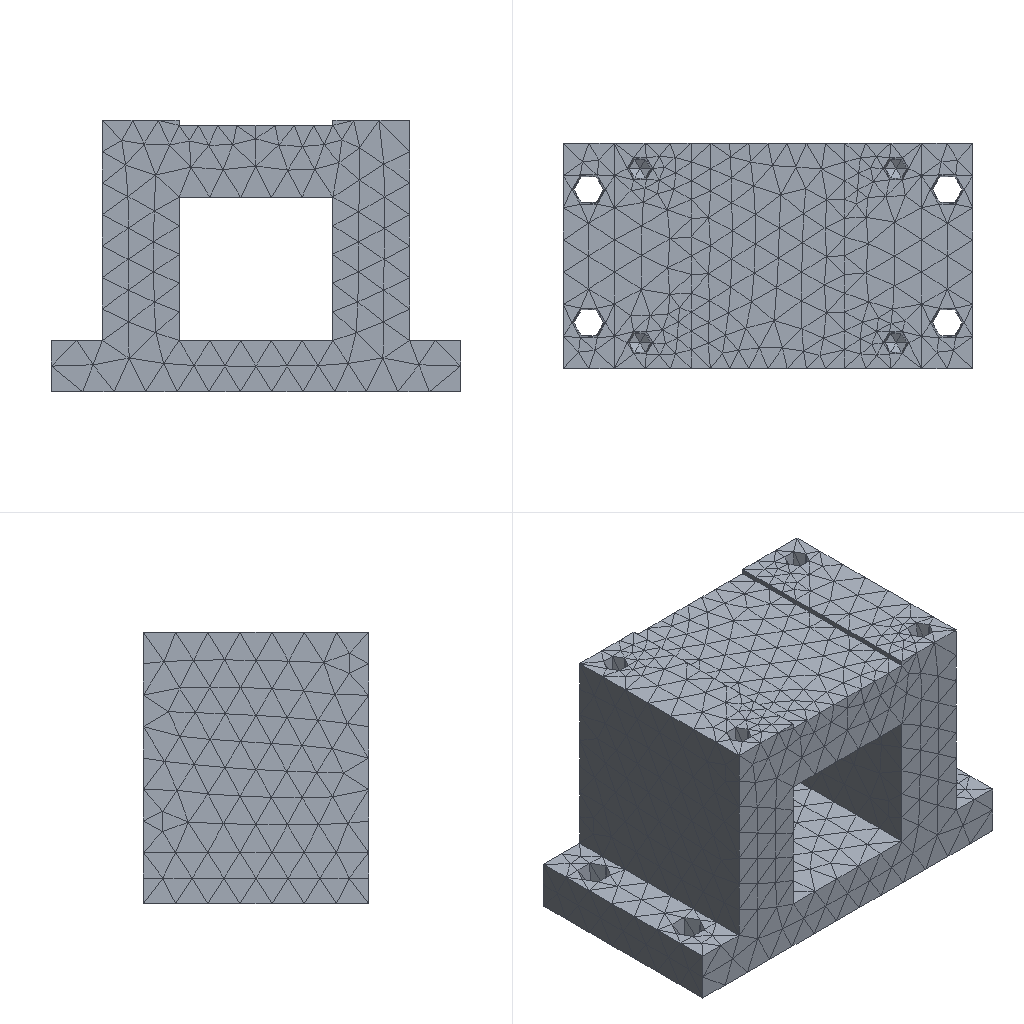Simulation study | nx simcenter
Set-up summary:
category,name,step,type,value,unit,region
solver,nx_nastran (Simcenter)
units,not stated in the deck,,not stated
analysis,deck,,static,static
analysis,solution,,SOL,101
load_step,SUBCASE 1,1,SUBCASE,SPC=1 LOAD=2
load_step,requested,,,1
mesh,nodes,,,7236
mesh,elements,,,3939
element_type,CTETRA,,solid,3939
load,nodal force total,,FX,0.0,model units
load,nodal force total,,FY,0.0,model units
load,nodal force total,,FZ,-3499999.96,model units
load,load commands in deck,,count,316
bc,support commands in deck,,count,569
analysis,NX solution 0,,Structural,Linear Statics - Single Constraint
check,setup vs results,,match,every grid point's frame and coordinates and every element id; grid points of CTETRA elements
Nastran input file, long lists of numbers shortened:
$*$$$$$$$$$$$$$$$$$$$$$$$$$$$$$$$$$$$$$$$$$$$$$$$$$$$$$$$$$$$$$$$$$
$*
$*                    NX v10.0.0.24 TRANSLATOR
$*                    FOR NX NASTRAN VERSION 10.0
$ (33 more lines like these left out)
ASSIGN OUTPUT2='157_sim1-solution_1.op2' UNIT=12
$*
$*$$$$$$$$$$$$$$$$$$$$$$$$$$$$$$$$$$$
$*
$* EXECUTIVE CONTROL
$*
$*$$$$$$$$$$$$$$$$$$$$$$$$$$$$$$$$$$$
$*
ID,NASTRAN,157_sim1-solution_1
SOL 101
CEND
$*
$*$$$$$$$$$$$$$$$$$$$$$$$$$$$$$$$$$$$
$*
$* CASE CONTROL
$*
$*$$$$$$$$$$$$$$$$$$$$$$$$$$$$$$$$$$$
$*
TITLE = Solution 1
ECHO = NONE
SPC = 1
OUTPUT
BCRESULTS(TRACTION,FORCE,PLOT) = ALL
DISPLACEMENT(PLOT) = ALL
ESE(PLOT) = ALL
FORCE(PLOT,CORNER) = ALL
OLOAD(PLOT) = ALL
SPCFORCES(PLOT) = ALL
STRAIN(PLOT,FIBER,CORNER) = ALL
STRESS(PLOT,CORNER) = ALL
$*  NX Step: Subcase - Static Loads 1
SUBCASE 1
LABEL = Subcase - Static Loads 1
LOAD = 2
$*
$*$$$$$$$$$$$$$$$$$$$$$$$$$$$$$$$$$$$
$*
$* BULK DATA
$*
$*$$$$$$$$$$$$$$$$$$$$$$$$$$$$$$$$$$$
$*
BEGIN BULK
$*
$* PARAM CARDS
$*
PARAM      K6ROT100.0000
PARAM     OIBULK     YES
PARAM    OMACHPR     YES
PARAM       POST      -2
PARAM    POSTEXT     YES
PARAM    UNITSYS   MN-MM
$*
$* GRID CARDS
$*
GRID*               7189               0-3.000000000E+01-4.400000000E+01+
*       2.2000000000E+01               0
GRID*               7190               0-3.000000000E+01-4.400000000E+01+
*       1.2000000000E+01               0
$ (14468 more lines like these left out)
$*
$* ELEMENT CARDS
$*
$*  NX Mesh Collector: Solid(1)
$*  NX Mesh: 3d_mesh(1)
CTETRA         1       1       1       2    3493    4848     217     218+
+            219     220     221     222
CTETRA         2       1       2       3    6670       1     223     224+
+            225     217     226     227
$ (7874 more lines like these left out)
$*
$* PROPERTY CARDS
$*
$*  NX Property: PSOLID1
PSOLID         1       1       0                           SMECH
$*
$* MATERIAL CARDS
$*
$*  NX Material: 2A12
MAT1           17.3119+7        0.3300002.8000-62.1355-5
MATT1          1       1               2               3
TABLEM1        1                                                        +
+        20.00007.3119+7 21.11007.3119+7 23.89007.3119+7 37.78007.3119+7+
+        51.67007.3119+7 65.56007.2429+7 79.44007.2429+7 93.33007.1739+7+
+       107.22007.1049+7121.11007.0359+7135.00006.9670+7148.89006.8980+7+
+       162.78006.8290+7176.67006.6910+7190.56006.6221+7204.44006.4841+7+
+       218.33006.3461+7232.22006.1392+7246.11006.0012+7260.00005.8633+7+
+       273.89005.7253+7287.78005.5184+7301.67005.3804+7315.56005.1735+7+
+       329.44004.9665+7343.33004.7596+7357.22004.6216+7371.11004.4147+7+
+           ENDT
TABLEM1        2                                                        +
+        20.00000.330000 21.11000.330000    ENDT
TABLEM1        3                                                        +
+        20.00002.1600-5 93.33002.2500-5107.22002.2662-5121.11002.2824-5+
+       135.00002.2968-5148.89002.3130-5162.78002.3274-5176.67002.3418-5+
+       190.56002.3544-5204.44002.3688-5218.33002.3814-5232.22002.3958-5+
+       246.11002.4066-5260.00002.4192-5273.89002.4300-5287.78002.4408-5+
+       301.67002.4498-5315.56002.4606-5329.44002.4696-5343.33002.4786-5+
+       357.22002.4876-5371.11002.4984-5385.00002.5110-5398.89002.5254-5+
+       412.78002.5398-5426.67002.5560-5    ENDT
$*
$* LOAD AND CONSTRAINT CARDS
$*
$*  NX Load and Constraint: Fixed(1)
SPC            1    5784  123456  0.0000
SPC            1    5785  123456  0.0000
SPC            1    5786  123456  0.0000
SPC            1    5787  123456  0.0000
$ (565 more lines like these left out)
$*  NX Load and Constraint: Force(1)
FORCE          2    3710       0 8254.55  0.0000  0.0000-1.00000
FORCE          2    3711       0 7399.16  0.0000  0.0000-1.00000
FORCE          2    3712       0 8557.39  0.0000  0.0000-1.00000
FORCE          2    3713       0 8804.06  0.0000  0.0000-1.00000
$ (312 more lines like these left out)
ENDDATA 84912eaa
Results summary:
result,analysis,,,static
result,last_loadstep,,,1
result,primary field,,,displacements
result,max displacement,,,0.001884,model units
result,reaction total,,FX,-0.05542,model units
result,reaction total,,FY,0.04224,model units
result,reaction total,,FZ,3499999.75,model units
result,NX solution 0,,loadcases,1,mm